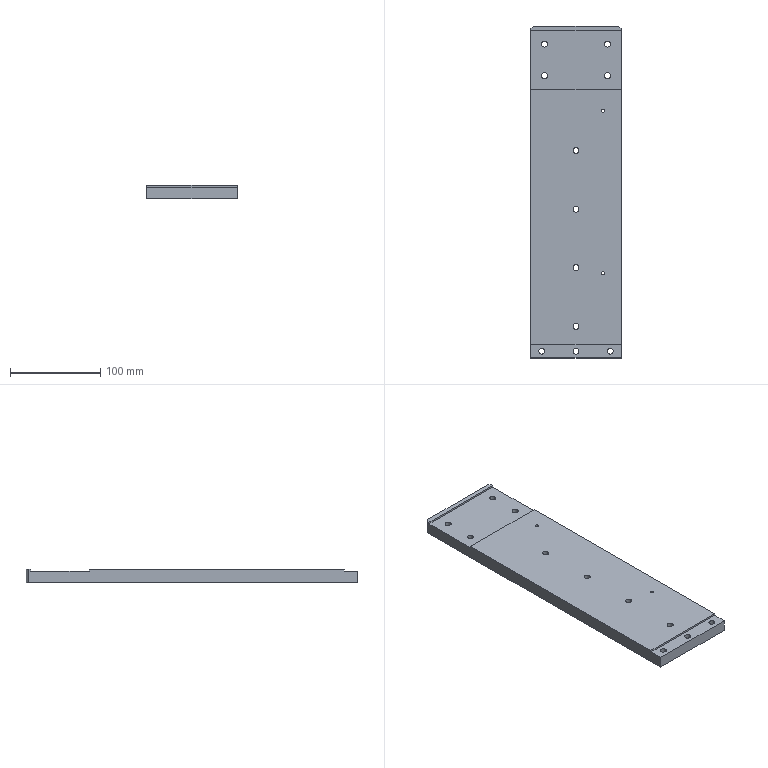Part | STEP file | PN_0018 | 1 solid | 73 faces | box 100 x 368 x 15 mm | volume 525873 mm3 | cylinder 48 | plane 25 | commonest cylinder face diameters 6.6 x22 11 x22 3.3 x4